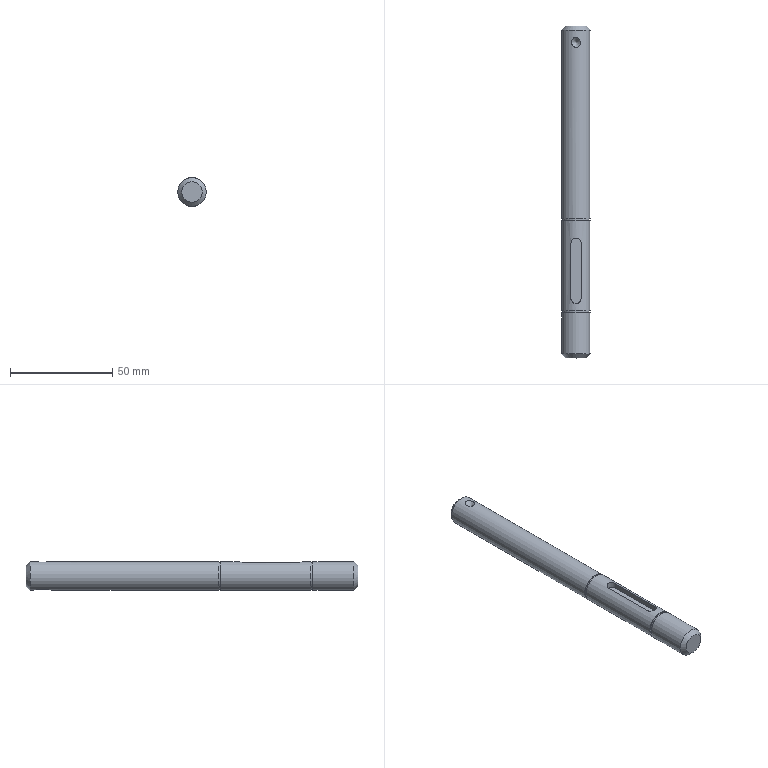Part | NX | features DATUM_CSYS 4, SKETCH 3, EXTRUDE 2, SWP104 2, CHAMFER 1, CYLINDER 1 | 1 solid | 24 faces | box 14 x 162 x 14 mm | volume 24153 mm3 | plane 12 | cylinder 9 | cone 3 | commonest cylinder face diameters 5 x4 14 x3 13 x2
STEP:
#1=CARTESIAN_POINT('',(0.,23.,-7.));
#2=VERTEX_POINT('',#1);
#3=CARTESIAN_POINT('',(0.,23.,0.));
#4=DIRECTION('',(0.,-1.,0.));
#5=DIRECTION('',(0.,0.,-1.));
#6=AXIS2_PLACEMENT_3D('',#3,#4,#5);
#7=CIRCLE('',#6,7.);
#8=EDGE_CURVE('',#2,#2,#7,.F.);
#9=ORIENTED_EDGE('',*,*,#8,.T.);
#10=EDGE_LOOP('',(#9));
#11=FACE_BOUND('',#10,.T.);
#12=CARTESIAN_POINT('',(0.,67.,7.));
#13=VERTEX_POINT('',#12);
#14=CARTESIAN_POINT('',(0.,67.,0.));
#15=DIRECTION('',(0.,1.,0.));
#16=DIRECTION('',(0.,0.,1.));
#17=AXIS2_PLACEMENT_3D('',#14,#15,#16);
#18=CIRCLE('',#17,7.);
#19=EDGE_CURVE('',#13,#13,#18,.F.);
#20=ORIENTED_EDGE('',*,*,#19,.T.);
#21=EDGE_LOOP('',(#20));
#22=FACE_BOUND('',#21,.T.);
#23=CARTESIAN_POINT('',(2.5,29.,6.538));
#24=VERTEX_POINT('',#23);
#25=CARTESIAN_POINT('',(-2.5,29.,6.538));
#26=VERTEX_POINT('',#25);
#27=CARTESIAN_POINT('',(2.5,29.,6.538));
#28=CARTESIAN_POINT('',(2.5,28.334,6.538));
#29=CARTESIAN_POINT('',(1.958,27.048,6.777));
#30=CARTESIAN_POINT('',(0.004587,26.226,7.111));
#31=CARTESIAN_POINT('',(-1.96,27.047,6.777));
#32=CARTESIAN_POINT('',(-2.5,28.333,6.538));
#33=CARTESIAN_POINT('',(-2.5,29.,6.538));
#34=B_SPLINE_CURVE_WITH_KNOTS('',3,(#27,#28,#29,#30,#31,#32,#33),.UNSPECIFIED.,.F.,.F.,(4,1,1,1,4),(0.,0.00197,0.003939,0.005909,0.007878),.UNSPECIFIED.);
#35=EDGE_CURVE('',#24,#26,#34,.T.);
#36=ORIENTED_EDGE('',*,*,#35,.T.);
#37=CARTESIAN_POINT('',(-2.5,56.,6.538));
#38=VERTEX_POINT('',#37);
#39=CARTESIAN_POINT('',(-2.5,0.,6.538));
#40=DIRECTION('',(0.,1.,0.));
#41=VECTOR('',#40,1000.);
#42=LINE('',#39,#41);
#43=EDGE_CURVE('',#26,#38,#42,.T.);
#44=ORIENTED_EDGE('',*,*,#43,.T.);
#45=CARTESIAN_POINT('',(2.5,56.,6.538));
#46=VERTEX_POINT('',#45);
#47=CARTESIAN_POINT('',(-2.5,56.,6.538));
#48=CARTESIAN_POINT('',(-2.5,56.666,6.538));
#49=CARTESIAN_POINT('',(-1.958,57.952,6.777));
#50=CARTESIAN_POINT('',(-0.004587,58.774,7.111));
#51=CARTESIAN_POINT('',(1.96,57.953,6.777));
#52=CARTESIAN_POINT('',(2.5,56.667,6.538));
#53=CARTESIAN_POINT('',(2.5,56.,6.538));
#54=B_SPLINE_CURVE_WITH_KNOTS('',3,(#47,#48,#49,#50,#51,#52,#53),.UNSPECIFIED.,.F.,.F.,(4,1,1,1,4),(0.,0.00197,0.003939,0.005909,0.007878),.UNSPECIFIED.);
#55=EDGE_CURVE('',#38,#46,#54,.T.);
#56=ORIENTED_EDGE('',*,*,#55,.T.);
#57=CARTESIAN_POINT('',(2.5,0.,6.538));
#58=DIRECTION('',(0.,1.,0.));
#59=VECTOR('',#58,1000.);
#60=LINE('',#57,#59);
#61=EDGE_CURVE('',#46,#24,#60,.F.);
#62=ORIENTED_EDGE('',*,*,#61,.T.);
#63=EDGE_LOOP('',(#36,#44,#56,#62));
#64=FACE_BOUND('',#63,.T.);
#65=CARTESIAN_POINT('',(0.,0.,0.));
#66=DIRECTION('',(0.,1.,0.));
#67=DIRECTION('',(1.,0.,0.));
#68=AXIS2_PLACEMENT_3D('',#65,#66,#67);
#69=CYLINDRICAL_SURFACE('',#68,7.);
#70=ADVANCED_FACE('',(#11,#22,#64),#69,.T.);
#71=CARTESIAN_POINT('',(-2.5,151.5,-6.538));
#72=VERTEX_POINT('',#71);
#73=CARTESIAN_POINT('',(-2.5,156.5,-6.538));
#74=VERTEX_POINT('',#73);
#75=CARTESIAN_POINT('',(-2.5,0.,-6.538));
#76=DIRECTION('',(0.,1.,0.));
#77=VECTOR('',#76,1000.);
#78=LINE('',#75,#77);
#79=EDGE_CURVE('',#72,#74,#78,.T.);
#80=ORIENTED_EDGE('',*,*,#79,.F.);
#81=CARTESIAN_POINT('',(2.5,151.5,-6.538));
#82=VERTEX_POINT('',#81);
#83=CARTESIAN_POINT('',(2.5,151.5,-6.538));
#84=CARTESIAN_POINT('',(2.5,150.834,-6.538));
#85=CARTESIAN_POINT('',(1.958,149.548,-6.777));
#86=CARTESIAN_POINT('',(0.004587,148.726,-7.111));
#87=CARTESIAN_POINT('',(-1.96,149.547,-6.777));
#88=CARTESIAN_POINT('',(-2.5,150.833,-6.538));
#89=CARTESIAN_POINT('',(-2.5,151.5,-6.538));
#90=B_SPLINE_CURVE_WITH_KNOTS('',3,(#83,#84,#85,#86,#87,#88,#89),.UNSPECIFIED.,.F.,.F.,(4,1,1,1,4),(0.,0.00197,0.003939,0.005909,0.007878),.UNSPECIFIED.);
#91=EDGE_CURVE('',#82,#72,#90,.T.);
#92=ORIENTED_EDGE('',*,*,#91,.F.);
#93=CARTESIAN_POINT('',(2.5,156.5,-6.538));
#94=VERTEX_POINT('',#93);
#95=CARTESIAN_POINT('',(2.5,0.,-6.538));
#96=DIRECTION('',(0.,1.,0.));
#97=VECTOR('',#96,1000.);
#98=LINE('',#95,#97);
#99=EDGE_CURVE('',#94,#82,#98,.F.);
#100=ORIENTED_EDGE('',*,*,#99,.F.);
#101=CARTESIAN_POINT('',(-2.5,156.5,-6.538));
#102=CARTESIAN_POINT('',(-2.5,157.166,-6.538));
#103=CARTESIAN_POINT('',(-1.958,158.452,-6.777));
#104=CARTESIAN_POINT('',(-0.004587,159.274,-7.111));
#105=CARTESIAN_POINT('',(1.96,158.453,-6.777));
#106=CARTESIAN_POINT('',(2.5,157.167,-6.538));
#107=CARTESIAN_POINT('',(2.5,156.5,-6.538));
#108=B_SPLINE_CURVE_WITH_KNOTS('',3,(#101,#102,#103,#104,#105,#106,#107),.UNSPECIFIED.,.F.,.F.,(4,1,1,1,4),(0.,0.00197,0.003939,0.005909,0.007878),.UNSPECIFIED.);
#109=EDGE_CURVE('',#74,#94,#108,.T.);
#110=ORIENTED_EDGE('',*,*,#109,.F.);
#111=EDGE_LOOP('',(#80,#92,#100,#110));
#112=FACE_BOUND('',#111,.T.);
#113=CARTESIAN_POINT('',(-1.745,152.535,6.779));
#114=VERTEX_POINT('',#113);
#115=CARTESIAN_POINT('',(-2.335,154.307,6.589));
#116=CARTESIAN_POINT('',(-1.947,152.424,6.75));
#117=CARTESIAN_POINT('',(-0.3497,151.204,7.084));
#118=CARTESIAN_POINT('',(1.577,151.902,6.875));
#119=CARTESIAN_POINT('',(2.333,153.69,6.59));
#120=CARTESIAN_POINT('',(1.952,155.566,6.748));
#121=CARTESIAN_POINT('',(0.3554,156.797,7.084));
#122=CARTESIAN_POINT('',(-1.576,156.1,6.875));
#123=CARTESIAN_POINT('',(-2.335,154.307,6.589));
#124=CARTESIAN_POINT('',(-1.947,152.424,6.75));
#125=CARTESIAN_POINT('',(-0.3497,151.204,7.084));
#126=B_SPLINE_CURVE_WITH_KNOTS('',3,(#115,#116,#117,#118,#119,#120,#121,#122,#123,#124,#125),.UNSPECIFIED.,.T.,.F.,(1,1,1,1,1,1,1,1,1,1,1,1,1,1,1),(-0.005507,-0.003671,-0.001836,0.,0.001836,0.003671,0.005507,0.007342,0.009178,0.01101,0.01285,0.01468,0.01652,0.01836,0.02019),.UNSPECIFIED.);
#127=EDGE_CURVE('',#114,#114,#126,.T.);
#128=ORIENTED_EDGE('',*,*,#127,.F.);
#129=EDGE_LOOP('',(#128));
#130=FACE_BOUND('',#129,.T.);
#131=CARTESIAN_POINT('',(0.,160.,7.));
#132=VERTEX_POINT('',#131);
#133=CARTESIAN_POINT('',(0.,160.,0.));
#134=DIRECTION('',(0.,1.,0.));
#135=DIRECTION('',(0.,0.,1.));
#136=AXIS2_PLACEMENT_3D('',#133,#134,#135);
#137=CIRCLE('',#136,7.);
#138=EDGE_CURVE('',#132,#132,#137,.F.);
#139=ORIENTED_EDGE('',*,*,#138,.T.);
#140=EDGE_LOOP('',(#139));
#141=FACE_BOUND('',#140,.T.);
#142=CARTESIAN_POINT('',(0.,68.,-7.));
#143=VERTEX_POINT('',#142);
#144=CARTESIAN_POINT('',(0.,68.,0.));
#145=DIRECTION('',(0.,-1.,0.));
#146=DIRECTION('',(0.,0.,-1.));
#147=AXIS2_PLACEMENT_3D('',#144,#145,#146);
#148=CIRCLE('',#147,7.);
#149=EDGE_CURVE('',#143,#143,#148,.F.);
#150=ORIENTED_EDGE('',*,*,#149,.T.);
#151=EDGE_LOOP('',(#150));
#152=FACE_BOUND('',#151,.T.);
#153=CARTESIAN_POINT('',(0.,0.,0.));
#154=DIRECTION('',(0.,1.,0.));
#155=DIRECTION('',(1.,0.,0.));
#156=AXIS2_PLACEMENT_3D('',#153,#154,#155);
#157=CYLINDRICAL_SURFACE('',#156,7.);
#158=ADVANCED_FACE('',(#112,#130,#141,#152),#157,.T.);
#159=CARTESIAN_POINT('',(0.,162.,5.));
#160=VERTEX_POINT('',#159);
#161=CARTESIAN_POINT('',(0.,162.,0.));
#162=DIRECTION('',(0.,1.,0.));
#163=DIRECTION('',(0.,0.,1.));
#164=AXIS2_PLACEMENT_3D('',#161,#162,#163);
#165=CIRCLE('',#164,5.);
#166=EDGE_CURVE('',#160,#160,#165,.T.);
#167=ORIENTED_EDGE('',*,*,#166,.T.);
#168=EDGE_LOOP('',(#167));
#169=FACE_BOUND('',#168,.T.);
#170=CARTESIAN_POINT('',(0.,162.,0.));
#171=DIRECTION('',(0.,1.,0.));
#172=DIRECTION('',(0.,0.,1.));
#173=AXIS2_PLACEMENT_3D('',#170,#171,#172);
#174=PLANE('',#173);
#175=ADVANCED_FACE('',(#169),#174,.T.);
#176=ORIENTED_EDGE('',*,*,#166,.F.);
#177=EDGE_LOOP('',(#176));
#178=FACE_BOUND('',#177,.T.);
#179=ORIENTED_EDGE('',*,*,#138,.F.);
#180=EDGE_LOOP('',(#179));
#181=FACE_BOUND('',#180,.T.);
#182=CARTESIAN_POINT('',(0.,160.,0.));
#183=DIRECTION('',(0.,-1.,0.));
#184=DIRECTION('',(0.,0.,-1.));
#185=AXIS2_PLACEMENT_3D('',#182,#183,#184);
#186=CONICAL_SURFACE('',#185,7.,0.7854);
#187=ADVANCED_FACE('',(#178,#181),#186,.T.);
#188=ORIENTED_EDGE('',*,*,#19,.F.);
#189=EDGE_LOOP('',(#188));
#190=FACE_BOUND('',#189,.T.);
#191=CARTESIAN_POINT('',(0.,67.,-6.5));
#192=VERTEX_POINT('',#191);
#193=CARTESIAN_POINT('',(0.,67.,0.));
#194=DIRECTION('',(0.,-1.,0.));
#195=DIRECTION('',(0.,0.,-1.));
#196=AXIS2_PLACEMENT_3D('',#193,#194,#195);
#197=CIRCLE('',#196,6.5);
#198=EDGE_CURVE('',#192,#192,#197,.F.);
#199=ORIENTED_EDGE('',*,*,#198,.F.);
#200=EDGE_LOOP('',(#199));
#201=FACE_BOUND('',#200,.T.);
#202=CARTESIAN_POINT('',(0.,67.,11.69));
#203=DIRECTION('',(0.,1.,0.));
#204=DIRECTION('',(0.,0.,1.));
#205=AXIS2_PLACEMENT_3D('',#202,#203,#204);
#206=PLANE('',#205);
#207=ADVANCED_FACE('',(#190,#201),#206,.T.);
#208=CARTESIAN_POINT('',(0.,68.,-6.5));
#209=VERTEX_POINT('',#208);
#210=CARTESIAN_POINT('',(0.,68.,0.));
#211=DIRECTION('',(0.,-1.,0.));
#212=DIRECTION('',(0.,0.,-1.));
#213=AXIS2_PLACEMENT_3D('',#210,#211,#212);
#214=CIRCLE('',#213,6.5);
#215=EDGE_CURVE('',#209,#209,#214,.F.);
#216=ORIENTED_EDGE('',*,*,#215,.F.);
#217=EDGE_LOOP('',(#216));
#218=FACE_BOUND('',#217,.T.);
#219=ORIENTED_EDGE('',*,*,#198,.T.);
#220=EDGE_LOOP('',(#219));
#221=FACE_BOUND('',#220,.T.);
#222=CARTESIAN_POINT('',(0.,0.,0.));
#223=DIRECTION('',(0.,-1.,0.));
#224=DIRECTION('',(0.,0.,-1.));
#225=AXIS2_PLACEMENT_3D('',#222,#223,#224);
#226=CYLINDRICAL_SURFACE('',#225,6.5);
#227=ADVANCED_FACE('',(#218,#221),#226,.T.);
#228=ORIENTED_EDGE('',*,*,#149,.F.);
#229=EDGE_LOOP('',(#228));
#230=FACE_BOUND('',#229,.T.);
#231=ORIENTED_EDGE('',*,*,#215,.T.);
#232=EDGE_LOOP('',(#231));
#233=FACE_BOUND('',#232,.T.);
#234=CARTESIAN_POINT('',(0.,68.,6.5));
#235=DIRECTION('',(0.,-1.,0.));
#236=DIRECTION('',(0.,0.,-1.));
#237=AXIS2_PLACEMENT_3D('',#234,#235,#236);
#238=PLANE('',#237);
#239=ADVANCED_FACE('',(#230,#233),#238,.T.);
#240=CARTESIAN_POINT('',(0.,22.,7.));
#241=VERTEX_POINT('',#240);
#242=CARTESIAN_POINT('',(0.,22.,0.));
#243=DIRECTION('',(0.,1.,0.));
#244=DIRECTION('',(0.,0.,1.));
#245=AXIS2_PLACEMENT_3D('',#242,#243,#244);
#246=CIRCLE('',#245,7.);
#247=EDGE_CURVE('',#241,#241,#246,.F.);
#248=ORIENTED_EDGE('',*,*,#247,.F.);
#249=EDGE_LOOP('',(#248));
#250=FACE_BOUND('',#249,.T.);
#251=CARTESIAN_POINT('',(0.,22.,-6.5));
#252=VERTEX_POINT('',#251);
#253=CARTESIAN_POINT('',(0.,22.,0.));
#254=DIRECTION('',(0.,-1.,0.));
#255=DIRECTION('',(0.,0.,-1.));
#256=AXIS2_PLACEMENT_3D('',#253,#254,#255);
#257=CIRCLE('',#256,6.5);
#258=EDGE_CURVE('',#252,#252,#257,.F.);
#259=ORIENTED_EDGE('',*,*,#258,.F.);
#260=EDGE_LOOP('',(#259));
#261=FACE_BOUND('',#260,.T.);
#262=CARTESIAN_POINT('',(0.,22.,14.266));
#263=DIRECTION('',(0.,1.,0.));
#264=DIRECTION('',(0.,0.,1.));
#265=AXIS2_PLACEMENT_3D('',#262,#263,#264);
#266=PLANE('',#265);
#267=ADVANCED_FACE('',(#250,#261),#266,.T.);
#268=CARTESIAN_POINT('',(0.,23.,-6.5));
#269=VERTEX_POINT('',#268);
#270=CARTESIAN_POINT('',(0.,23.,0.));
#271=DIRECTION('',(0.,-1.,0.));
#272=DIRECTION('',(0.,0.,-1.));
#273=AXIS2_PLACEMENT_3D('',#270,#271,#272);
#274=CIRCLE('',#273,6.5);
#275=EDGE_CURVE('',#269,#269,#274,.F.);
#276=ORIENTED_EDGE('',*,*,#275,.F.);
#277=EDGE_LOOP('',(#276));
#278=FACE_BOUND('',#277,.T.);
#279=ORIENTED_EDGE('',*,*,#258,.T.);
#280=EDGE_LOOP('',(#279));
#281=FACE_BOUND('',#280,.T.);
#282=CARTESIAN_POINT('',(0.,0.,0.));
#283=DIRECTION('',(0.,-1.,0.));
#284=DIRECTION('',(0.,0.,-1.));
#285=AXIS2_PLACEMENT_3D('',#282,#283,#284);
#286=CYLINDRICAL_SURFACE('',#285,6.5);
#287=ADVANCED_FACE('',(#278,#281),#286,.T.);
#288=ORIENTED_EDGE('',*,*,#8,.F.);
#289=EDGE_LOOP('',(#288));
#290=FACE_BOUND('',#289,.T.);
#291=ORIENTED_EDGE('',*,*,#275,.T.);
#292=EDGE_LOOP('',(#291));
#293=FACE_BOUND('',#292,.T.);
#294=CARTESIAN_POINT('',(0.,23.,6.5));
#295=DIRECTION('',(0.,-1.,0.));
#296=DIRECTION('',(0.,0.,-1.));
#297=AXIS2_PLACEMENT_3D('',#294,#295,#296);
#298=PLANE('',#297);
#299=ADVANCED_FACE('',(#290,#293),#298,.T.);
#300=CARTESIAN_POINT('',(0.,0.,-5.));
#301=VERTEX_POINT('',#300);
#302=CARTESIAN_POINT('',(0.,0.,0.));
#303=DIRECTION('',(0.,-1.,0.));
#304=DIRECTION('',(0.,0.,-1.));
#305=AXIS2_PLACEMENT_3D('',#302,#303,#304);
#306=CIRCLE('',#305,5.);
#307=EDGE_CURVE('',#301,#301,#306,.T.);
#308=ORIENTED_EDGE('',*,*,#307,.T.);
#309=EDGE_LOOP('',(#308));
#310=FACE_BOUND('',#309,.T.);
#311=CARTESIAN_POINT('',(0.,0.,0.));
#312=DIRECTION('',(0.,-1.,0.));
#313=DIRECTION('',(0.,0.,-1.));
#314=AXIS2_PLACEMENT_3D('',#311,#312,#313);
#315=PLANE('',#314);
#316=ADVANCED_FACE('',(#310),#315,.T.);
#317=ORIENTED_EDGE('',*,*,#307,.F.);
#318=EDGE_LOOP('',(#317));
#319=FACE_BOUND('',#318,.T.);
#320=CARTESIAN_POINT('',(0.,2.,-7.));
#321=VERTEX_POINT('',#320);
#322=CARTESIAN_POINT('',(0.,2.,0.));
#323=DIRECTION('',(0.,-1.,0.));
#324=DIRECTION('',(0.,0.,-1.));
#325=AXIS2_PLACEMENT_3D('',#322,#323,#324);
#326=CIRCLE('',#325,7.);
#327=EDGE_CURVE('',#321,#321,#326,.F.);
#328=ORIENTED_EDGE('',*,*,#327,.F.);
#329=EDGE_LOOP('',(#328));
#330=FACE_BOUND('',#329,.T.);
#331=CARTESIAN_POINT('',(0.,2.,0.));
#332=DIRECTION('',(0.,1.,0.));
#333=DIRECTION('',(0.,0.,1.));
#334=AXIS2_PLACEMENT_3D('',#331,#332,#333);
#335=CONICAL_SURFACE('',#334,7.,0.7854);
#336=ADVANCED_FACE('',(#319,#330),#335,.T.);
#337=ORIENTED_EDGE('',*,*,#327,.T.);
#338=EDGE_LOOP('',(#337));
#339=FACE_BOUND('',#338,.T.);
#340=ORIENTED_EDGE('',*,*,#247,.T.);
#341=EDGE_LOOP('',(#340));
#342=FACE_BOUND('',#341,.T.);
#343=CARTESIAN_POINT('',(0.,0.,0.));
#344=DIRECTION('',(0.,1.,0.));
#345=DIRECTION('',(1.,0.,0.));
#346=AXIS2_PLACEMENT_3D('',#343,#344,#345);
#347=CYLINDRICAL_SURFACE('',#346,7.);
#348=ADVANCED_FACE('',(#339,#342),#347,.T.);
#349=ORIENTED_EDGE('',*,*,#127,.T.);
#350=EDGE_LOOP('',(#349));
#351=FACE_BOUND('',#350,.T.);
#352=CARTESIAN_POINT('',(0.,154.,4.5));
#353=VERTEX_POINT('',#352);
#354=VERTEX_LOOP('',#353);
#355=FACE_BOUND('',#354,.T.);
#356=CARTESIAN_POINT('',(0.,154.,4.5));
#357=DIRECTION('',(0.,0.,1.));
#358=DIRECTION('',(1.,0.,0.));
#359=AXIS2_PLACEMENT_3D('',#356,#357,#358);
#360=CONICAL_SURFACE('',#359,0.,0.7854);
#361=ADVANCED_FACE('',(#351,#355),#360,.F.);
#362=CARTESIAN_POINT('',(-2.5,29.,4.));
#363=VERTEX_POINT('',#362);
#364=CARTESIAN_POINT('',(-2.5,29.,12.));
#365=DIRECTION('',(0.,0.,-1.));
#366=VECTOR('',#365,1000.);
#367=LINE('',#364,#366);
#368=EDGE_CURVE('',#363,#26,#367,.F.);
#369=ORIENTED_EDGE('',*,*,#368,.F.);
#370=CARTESIAN_POINT('',(-2.5,56.,4.));
#371=VERTEX_POINT('',#370);
#372=CARTESIAN_POINT('',(-2.5,56.,4.));
#373=DIRECTION('',(0.,-1.,0.));
#374=VECTOR('',#373,1000.);
#375=LINE('',#372,#374);
#376=EDGE_CURVE('',#363,#371,#375,.F.);
#377=ORIENTED_EDGE('',*,*,#376,.T.);
#378=CARTESIAN_POINT('',(-2.5,56.,12.));
#379=DIRECTION('',(0.,0.,-1.));
#380=VECTOR('',#379,1000.);
#381=LINE('',#378,#380);
#382=EDGE_CURVE('',#371,#38,#381,.F.);
#383=ORIENTED_EDGE('',*,*,#382,.T.);
#384=ORIENTED_EDGE('',*,*,#43,.F.);
#385=EDGE_LOOP('',(#369,#377,#383,#384));
#386=FACE_BOUND('',#385,.T.);
#387=CARTESIAN_POINT('',(-2.5,56.,12.));
#388=DIRECTION('',(1.,0.,0.));
#389=DIRECTION('',(0.,1.,0.));
#390=AXIS2_PLACEMENT_3D('',#387,#388,#389);
#391=PLANE('',#390);
#392=ADVANCED_FACE('',(#386),#391,.T.);
#393=CARTESIAN_POINT('',(2.5,29.,4.));
#394=VERTEX_POINT('',#393);
#395=CARTESIAN_POINT('',(2.5,29.,12.));
#396=DIRECTION('',(0.,0.,-1.));
#397=VECTOR('',#396,1000.);
#398=LINE('',#395,#397);
#399=EDGE_CURVE('',#394,#24,#398,.F.);
#400=ORIENTED_EDGE('',*,*,#399,.F.);
#401=CARTESIAN_POINT('',(0.,29.,4.));
#402=DIRECTION('',(0.,0.,1.));
#403=DIRECTION('',(1.,0.,0.));
#404=AXIS2_PLACEMENT_3D('',#401,#402,#403);
#405=CIRCLE('',#404,2.5);
#406=EDGE_CURVE('',#394,#363,#405,.F.);
#407=ORIENTED_EDGE('',*,*,#406,.T.);
#408=ORIENTED_EDGE('',*,*,#368,.T.);
#409=ORIENTED_EDGE('',*,*,#35,.F.);
#410=EDGE_LOOP('',(#400,#407,#408,#409));
#411=FACE_BOUND('',#410,.T.);
#412=CARTESIAN_POINT('',(0.,29.,12.));
#413=DIRECTION('',(0.,0.,-1.));
#414=DIRECTION('',(-1.,0.,0.));
#415=AXIS2_PLACEMENT_3D('',#412,#413,#414);
#416=CYLINDRICAL_SURFACE('',#415,2.5);
#417=ADVANCED_FACE('',(#411),#416,.F.);
#418=CARTESIAN_POINT('',(2.5,56.,4.));
#419=VERTEX_POINT('',#418);
#420=CARTESIAN_POINT('',(2.5,56.,12.));
#421=DIRECTION('',(0.,0.,-1.));
#422=VECTOR('',#421,1000.);
#423=LINE('',#420,#422);
#424=EDGE_CURVE('',#419,#46,#423,.F.);
#425=ORIENTED_EDGE('',*,*,#424,.F.);
#426=CARTESIAN_POINT('',(2.5,29.,4.));
#427=DIRECTION('',(0.,1.,0.));
#428=VECTOR('',#427,1000.);
#429=LINE('',#426,#428);
#430=EDGE_CURVE('',#419,#394,#429,.F.);
#431=ORIENTED_EDGE('',*,*,#430,.T.);
#432=ORIENTED_EDGE('',*,*,#399,.T.);
#433=ORIENTED_EDGE('',*,*,#61,.F.);
#434=EDGE_LOOP('',(#425,#431,#432,#433));
#435=FACE_BOUND('',#434,.T.);
#436=CARTESIAN_POINT('',(2.5,29.,12.));
#437=DIRECTION('',(-1.,0.,0.));
#438=DIRECTION('',(0.,-1.,0.));
#439=AXIS2_PLACEMENT_3D('',#436,#437,#438);
#440=PLANE('',#439);
#441=ADVANCED_FACE('',(#435),#440,.T.);
#442=ORIENTED_EDGE('',*,*,#382,.F.);
#443=CARTESIAN_POINT('',(0.,56.,4.));
#444=DIRECTION('',(0.,0.,1.));
#445=DIRECTION('',(1.,0.,0.));
#446=AXIS2_PLACEMENT_3D('',#443,#444,#445);
#447=CIRCLE('',#446,2.5);
#448=EDGE_CURVE('',#371,#419,#447,.F.);
#449=ORIENTED_EDGE('',*,*,#448,.T.);
#450=ORIENTED_EDGE('',*,*,#424,.T.);
#451=ORIENTED_EDGE('',*,*,#55,.F.);
#452=EDGE_LOOP('',(#442,#449,#450,#451));
#453=FACE_BOUND('',#452,.T.);
#454=CARTESIAN_POINT('',(0.,56.,12.));
#455=DIRECTION('',(0.,0.,-1.));
#456=DIRECTION('',(-1.,0.,0.));
#457=AXIS2_PLACEMENT_3D('',#454,#455,#456);
#458=CYLINDRICAL_SURFACE('',#457,2.5);
#459=ADVANCED_FACE('',(#453),#458,.F.);
#460=ORIENTED_EDGE('',*,*,#376,.F.);
#461=ORIENTED_EDGE('',*,*,#406,.F.);
#462=ORIENTED_EDGE('',*,*,#430,.F.);
#463=ORIENTED_EDGE('',*,*,#448,.F.);
#464=EDGE_LOOP('',(#460,#461,#462,#463));
#465=FACE_BOUND('',#464,.T.);
#466=CARTESIAN_POINT('',(0.,29.,4.));
#467=DIRECTION('',(0.,0.,1.));
#468=DIRECTION('',(1.,0.,0.));
#469=AXIS2_PLACEMENT_3D('',#466,#467,#468);
#470=PLANE('',#469);
#471=ADVANCED_FACE('',(#465),#470,.T.);
#472=ORIENTED_EDGE('',*,*,#79,.T.);
#473=CARTESIAN_POINT('',(-2.5,156.5,-4.));
#474=VERTEX_POINT('',#473);
#475=CARTESIAN_POINT('',(-2.5,156.5,-12.));
#476=DIRECTION('',(0.,0.,1.));
#477=VECTOR('',#476,1000.);
#478=LINE('',#475,#477);
#479=EDGE_CURVE('',#474,#74,#478,.F.);
#480=ORIENTED_EDGE('',*,*,#479,.F.);
#481=CARTESIAN_POINT('',(-2.5,151.5,-4.));
#482=VERTEX_POINT('',#481);
#483=CARTESIAN_POINT('',(-2.5,156.5,-4.));
#484=DIRECTION('',(0.,-1.,0.));
#485=VECTOR('',#484,1000.);
#486=LINE('',#483,#485);
#487=EDGE_CURVE('',#482,#474,#486,.F.);
#488=ORIENTED_EDGE('',*,*,#487,.F.);
#489=CARTESIAN_POINT('',(-2.5,151.5,-12.));
#490=DIRECTION('',(0.,0.,1.));
#491=VECTOR('',#490,1000.);
#492=LINE('',#489,#491);
#493=EDGE_CURVE('',#482,#72,#492,.F.);
#494=ORIENTED_EDGE('',*,*,#493,.T.);
#495=EDGE_LOOP('',(#472,#480,#488,#494));
#496=FACE_BOUND('',#495,.T.);
#497=CARTESIAN_POINT('',(-2.5,156.5,-12.));
#498=DIRECTION('',(-1.,0.,0.));
#499=DIRECTION('',(0.,-1.,0.));
#500=AXIS2_PLACEMENT_3D('',#497,#498,#499);
#501=PLANE('',#500);
#502=ADVANCED_FACE('',(#496),#501,.F.);
#503=ORIENTED_EDGE('',*,*,#91,.T.);
#504=ORIENTED_EDGE('',*,*,#493,.F.);
#505=CARTESIAN_POINT('',(2.5,151.5,-4.));
#506=VERTEX_POINT('',#505);
#507=CARTESIAN_POINT('',(0.,151.5,-4.));
#508=DIRECTION('',(0.,0.,1.));
#509=DIRECTION('',(1.,0.,0.));
#510=AXIS2_PLACEMENT_3D('',#507,#508,#509);
#511=CIRCLE('',#510,2.5);
#512=EDGE_CURVE('',#506,#482,#511,.F.);
#513=ORIENTED_EDGE('',*,*,#512,.F.);
#514=CARTESIAN_POINT('',(2.5,151.5,-12.));
#515=DIRECTION('',(0.,0.,1.));
#516=VECTOR('',#515,1000.);
#517=LINE('',#514,#516);
#518=EDGE_CURVE('',#506,#82,#517,.F.);
#519=ORIENTED_EDGE('',*,*,#518,.T.);
#520=EDGE_LOOP('',(#503,#504,#513,#519));
#521=FACE_BOUND('',#520,.T.);
#522=CARTESIAN_POINT('',(0.,151.5,-12.));
#523=DIRECTION('',(0.,0.,1.));
#524=DIRECTION('',(1.,0.,0.));
#525=AXIS2_PLACEMENT_3D('',#522,#523,#524);
#526=CYLINDRICAL_SURFACE('',#525,2.5);
#527=ADVANCED_FACE('',(#521),#526,.F.);
#528=ORIENTED_EDGE('',*,*,#99,.T.);
#529=ORIENTED_EDGE('',*,*,#518,.F.);
#530=CARTESIAN_POINT('',(2.5,156.5,-4.));
#531=VERTEX_POINT('',#530);
#532=CARTESIAN_POINT('',(2.5,151.5,-4.));
#533=DIRECTION('',(0.,1.,0.));
#534=VECTOR('',#533,1000.);
#535=LINE('',#532,#534);
#536=EDGE_CURVE('',#531,#506,#535,.F.);
#537=ORIENTED_EDGE('',*,*,#536,.F.);
#538=CARTESIAN_POINT('',(2.5,156.5,-12.));
#539=DIRECTION('',(0.,0.,1.));
#540=VECTOR('',#539,1000.);
#541=LINE('',#538,#540);
#542=EDGE_CURVE('',#531,#94,#541,.F.);
#543=ORIENTED_EDGE('',*,*,#542,.T.);
#544=EDGE_LOOP('',(#528,#529,#537,#543));
#545=FACE_BOUND('',#544,.T.);
#546=CARTESIAN_POINT('',(2.5,151.5,-12.));
#547=DIRECTION('',(1.,0.,0.));
#548=DIRECTION('',(0.,1.,0.));
#549=AXIS2_PLACEMENT_3D('',#546,#547,#548);
#550=PLANE('',#549);
#551=ADVANCED_FACE('',(#545),#550,.F.);
#552=ORIENTED_EDGE('',*,*,#109,.T.);
#553=ORIENTED_EDGE('',*,*,#542,.F.);
#554=CARTESIAN_POINT('',(0.,156.5,-4.));
#555=DIRECTION('',(0.,0.,1.));
#556=DIRECTION('',(1.,0.,0.));
#557=AXIS2_PLACEMENT_3D('',#554,#555,#556);
#558=CIRCLE('',#557,2.5);
#559=EDGE_CURVE('',#474,#531,#558,.F.);
#560=ORIENTED_EDGE('',*,*,#559,.F.);
#561=ORIENTED_EDGE('',*,*,#479,.T.);
#562=EDGE_LOOP('',(#552,#553,#560,#561));
#563=FACE_BOUND('',#562,.T.);
#564=CARTESIAN_POINT('',(0.,156.5,-12.));
#565=DIRECTION('',(0.,0.,1.));
#566=DIRECTION('',(1.,0.,0.));
#567=AXIS2_PLACEMENT_3D('',#564,#565,#566);
#568=CYLINDRICAL_SURFACE('',#567,2.5);
#569=ADVANCED_FACE('',(#563),#568,.F.);
#570=ORIENTED_EDGE('',*,*,#487,.T.);
#571=ORIENTED_EDGE('',*,*,#559,.T.);
#572=ORIENTED_EDGE('',*,*,#536,.T.);
#573=ORIENTED_EDGE('',*,*,#512,.T.);
#574=EDGE_LOOP('',(#570,#571,#572,#573));
#575=FACE_BOUND('',#574,.T.);
#576=CARTESIAN_POINT('',(0.,151.5,-4.));
#577=DIRECTION('',(0.,0.,1.));
#578=DIRECTION('',(1.,0.,0.));
#579=AXIS2_PLACEMENT_3D('',#576,#577,#578);
#580=PLANE('',#579);
#581=ADVANCED_FACE('',(#575),#580,.F.);
#582=CLOSED_SHELL('',(#70,#158,#175,#187,#207,#227,#239,#267,#287,#299,#316,#336,#348,#361,#392,#417,#441,#459,#471,#502,#527,#551,#569,#581));
#583=MANIFOLD_SOLID_BREP('',#582);
#584=(LENGTH_UNIT()NAMED_UNIT(*)SI_UNIT(.MILLI.,.METRE.));
#585=UNCERTAINTY_MEASURE_WITH_UNIT(LENGTH_MEASURE(0.0508),#584,'','');
#586=(NAMED_UNIT(*)PLANE_ANGLE_UNIT()SI_UNIT($,.RADIAN.));
#587=(NAMED_UNIT(*)SI_UNIT($,.STERADIAN.)SOLID_ANGLE_UNIT());
#588=(GEOMETRIC_REPRESENTATION_CONTEXT(3)GLOBAL_UNCERTAINTY_ASSIGNED_CONTEXT((#585))GLOBAL_UNIT_ASSIGNED_CONTEXT((#584,#586,#587))REPRESENTATION_CONTEXT('',''));
#589=ADVANCED_BREP_SHAPE_REPRESENTATION('',(#583),#588);